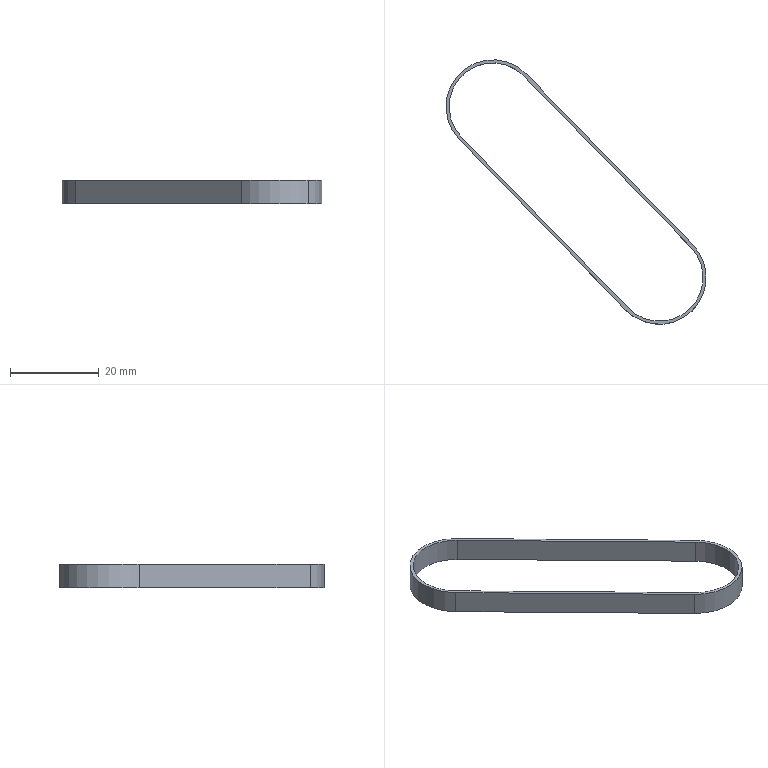Part | SolidWorks | features SplitBody 1 | 1 solid | 12 faces | box 58.599 x 59.577 x 5.25 mm | volume 630.396 mm3 | cylinder 6 | plane 6 | commonest cylinder face diameters 19.677 x3 21.077 x3
STEP:
#1=CARTESIAN_POINT('',(-26.957,211.226,-241.916));
#2=VERTEX_POINT('',#1);
#3=CARTESIAN_POINT('',(-27.136,197.313,-241.916));
#4=VERTEX_POINT('',#3);
#5=CARTESIAN_POINT('',(-34.003,204.359,-241.916));
#6=DIRECTION('',(0.,0.,-1.));
#7=DIRECTION('',(-0.698,0.7161,0.));
#8=AXIS2_PLACEMENT_3D('',#5,#6,#7);
#9=CIRCLE('',#8,9.838);
#10=EDGE_CURVE('',#2,#4,#9,.T.);
#11=ORIENTED_EDGE('',*,*,#10,.T.);
#12=CARTESIAN_POINT('',(-27.136,197.313,-236.666));
#13=VERTEX_POINT('',#12);
#14=CARTESIAN_POINT('',(-27.136,197.313,-241.916));
#15=DIRECTION('',(0.,0.,1.));
#16=VECTOR('',#15,1000.);
#17=LINE('',#14,#16);
#18=EDGE_CURVE('',#4,#13,#17,.T.);
#19=ORIENTED_EDGE('',*,*,#18,.T.);
#20=CARTESIAN_POINT('',(-26.957,211.226,-236.666));
#21=VERTEX_POINT('',#20);
#22=CARTESIAN_POINT('',(-34.003,204.359,-236.666));
#23=DIRECTION('',(0.,0.,-1.));
#24=DIRECTION('',(-0.698,0.7161,0.));
#25=AXIS2_PLACEMENT_3D('',#22,#23,#24);
#26=CIRCLE('',#25,9.838);
#27=EDGE_CURVE('',#21,#13,#26,.T.);
#28=ORIENTED_EDGE('',*,*,#27,.F.);
#29=CARTESIAN_POINT('',(-26.957,211.226,-241.916));
#30=DIRECTION('',(0.,0.,1.));
#31=VECTOR('',#30,1000.);
#32=LINE('',#29,#31);
#33=EDGE_CURVE('',#2,#21,#32,.T.);
#34=ORIENTED_EDGE('',*,*,#33,.F.);
#35=EDGE_LOOP('',(#11,#19,#28,#34));
#36=FACE_OUTER_BOUND('',#35,.T.);
#37=CARTESIAN_POINT('',(-34.003,204.359,-241.916));
#38=DIRECTION('',(0.,0.,1.));
#39=DIRECTION('',(0.698,-0.7161,0.));
#40=AXIS2_PLACEMENT_3D('',#37,#38,#39);
#41=CYLINDRICAL_SURFACE('',#40,9.838);
#42=ADVANCED_FACE('',(#36),#41,.F.);
#43=CARTESIAN_POINT('',(-26.648,196.812,-241.916));
#44=VERTEX_POINT('',#43);
#45=CARTESIAN_POINT('',(-41.55,197.004,-241.916));
#46=VERTEX_POINT('',#45);
#47=CARTESIAN_POINT('',(-34.003,204.359,-241.916));
#48=DIRECTION('',(0.,0.,-1.));
#49=DIRECTION('',(-0.698,0.7161,0.));
#50=AXIS2_PLACEMENT_3D('',#47,#48,#49);
#51=CIRCLE('',#50,10.538);
#52=EDGE_CURVE('',#44,#46,#51,.T.);
#53=ORIENTED_EDGE('',*,*,#52,.F.);
#54=CARTESIAN_POINT('',(-26.648,196.812,-236.666));
#55=VERTEX_POINT('',#54);
#56=CARTESIAN_POINT('',(-26.648,196.812,-241.916));
#57=DIRECTION('',(0.,0.,1.));
#58=VECTOR('',#57,1000.);
#59=LINE('',#56,#58);
#60=EDGE_CURVE('',#44,#55,#59,.T.);
#61=ORIENTED_EDGE('',*,*,#60,.T.);
#62=CARTESIAN_POINT('',(-41.55,197.004,-236.666));
#63=VERTEX_POINT('',#62);
#64=CARTESIAN_POINT('',(-34.003,204.359,-236.666));
#65=DIRECTION('',(0.,0.,-1.));
#66=DIRECTION('',(-0.698,0.7161,0.));
#67=AXIS2_PLACEMENT_3D('',#64,#65,#66);
#68=CIRCLE('',#67,10.538);
#69=EDGE_CURVE('',#55,#63,#68,.T.);
#70=ORIENTED_EDGE('',*,*,#69,.T.);
#71=CARTESIAN_POINT('',(-41.55,197.004,-241.916));
#72=DIRECTION('',(0.,0.,1.));
#73=VECTOR('',#72,1000.);
#74=LINE('',#71,#73);
#75=EDGE_CURVE('',#46,#63,#74,.T.);
#76=ORIENTED_EDGE('',*,*,#75,.F.);
#77=EDGE_LOOP('',(#53,#61,#70,#76));
#78=FACE_OUTER_BOUND('',#77,.T.);
#79=CARTESIAN_POINT('',(-34.003,204.359,-241.916));
#80=DIRECTION('',(0.,0.,1.));
#81=DIRECTION('',(0.698,-0.7161,0.));
#82=AXIS2_PLACEMENT_3D('',#79,#80,#81);
#83=CYLINDRICAL_SURFACE('',#82,10.538);
#84=ADVANCED_FACE('',(#78),#83,.T.);
#85=CARTESIAN_POINT('',(-26.456,211.714,-241.916));
#86=VERTEX_POINT('',#85);
#87=CARTESIAN_POINT('',(-34.003,204.359,-241.916));
#88=DIRECTION('',(0.,0.,-1.));
#89=DIRECTION('',(-0.698,0.7161,0.));
#90=AXIS2_PLACEMENT_3D('',#87,#88,#89);
#91=CIRCLE('',#90,10.538);
#92=EDGE_CURVE('',#86,#44,#91,.T.);
#93=ORIENTED_EDGE('',*,*,#92,.T.);
#94=ORIENTED_EDGE('',*,*,#52,.T.);
#95=CARTESIAN_POINT('',(-79.072,235.504,-241.916));
#96=VERTEX_POINT('',#95);
#97=CARTESIAN_POINT('',(-79.072,235.504,-241.916));
#98=DIRECTION('',(-0.698,0.7161,0.));
#99=VECTOR('',#98,1000.);
#100=LINE('',#97,#99);
#101=EDGE_CURVE('',#46,#96,#100,.T.);
#102=ORIENTED_EDGE('',*,*,#101,.T.);
#103=CARTESIAN_POINT('',(-63.978,250.214,-241.916));
#104=VERTEX_POINT('',#103);
#105=CARTESIAN_POINT('',(-71.525,242.859,-241.916));
#106=DIRECTION('',(0.,0.,-1.));
#107=DIRECTION('',(-0.698,0.7161,0.));
#108=AXIS2_PLACEMENT_3D('',#105,#106,#107);
#109=CIRCLE('',#108,10.538);
#110=EDGE_CURVE('',#96,#104,#109,.T.);
#111=ORIENTED_EDGE('',*,*,#110,.T.);
#112=CARTESIAN_POINT('',(-26.456,211.714,-241.916));
#113=DIRECTION('',(0.698,-0.7161,0.));
#114=VECTOR('',#113,1000.);
#115=LINE('',#112,#114);
#116=EDGE_CURVE('',#104,#86,#115,.T.);
#117=ORIENTED_EDGE('',*,*,#116,.T.);
#118=EDGE_LOOP('',(#93,#94,#102,#111,#117));
#119=FACE_OUTER_BOUND('',#118,.T.);
#120=CARTESIAN_POINT('',(-41.049,197.492,-241.916));
#121=VERTEX_POINT('',#120);
#122=CARTESIAN_POINT('',(-78.57,235.992,-241.916));
#123=VERTEX_POINT('',#122);
#124=CARTESIAN_POINT('',(-78.57,235.992,-241.916));
#125=DIRECTION('',(-0.698,0.7161,0.));
#126=VECTOR('',#125,1000.);
#127=LINE('',#124,#126);
#128=EDGE_CURVE('',#121,#123,#127,.T.);
#129=ORIENTED_EDGE('',*,*,#128,.F.);
#130=CARTESIAN_POINT('',(-34.003,204.359,-241.916));
#131=DIRECTION('',(0.,0.,-1.));
#132=DIRECTION('',(-0.698,0.7161,0.));
#133=AXIS2_PLACEMENT_3D('',#130,#131,#132);
#134=CIRCLE('',#133,9.838);
#135=EDGE_CURVE('',#4,#121,#134,.T.);
#136=ORIENTED_EDGE('',*,*,#135,.F.);
#137=ORIENTED_EDGE('',*,*,#10,.F.);
#138=CARTESIAN_POINT('',(-64.479,249.726,-241.916));
#139=VERTEX_POINT('',#138);
#140=CARTESIAN_POINT('',(-26.957,211.226,-241.916));
#141=DIRECTION('',(0.698,-0.7161,0.));
#142=VECTOR('',#141,1000.);
#143=LINE('',#140,#142);
#144=EDGE_CURVE('',#139,#2,#143,.T.);
#145=ORIENTED_EDGE('',*,*,#144,.F.);
#146=CARTESIAN_POINT('',(-71.525,242.859,-241.916));
#147=DIRECTION('',(0.,0.,-1.));
#148=DIRECTION('',(-0.698,0.7161,0.));
#149=AXIS2_PLACEMENT_3D('',#146,#147,#148);
#150=CIRCLE('',#149,9.838);
#151=EDGE_CURVE('',#123,#139,#150,.T.);
#152=ORIENTED_EDGE('',*,*,#151,.F.);
#153=EDGE_LOOP('',(#129,#136,#137,#145,#152));
#154=FACE_BOUND('',#153,.T.);
#155=CARTESIAN_POINT('',(-34.003,204.359,-241.916));
#156=DIRECTION('',(0.,0.,-1.));
#157=DIRECTION('',(-0.698,0.7161,0.));
#158=AXIS2_PLACEMENT_3D('',#155,#156,#157);
#159=PLANE('',#158);
#160=ADVANCED_FACE('',(#119,#154),#159,.T.);
#161=CARTESIAN_POINT('',(-26.456,211.714,-236.666));
#162=VERTEX_POINT('',#161);
#163=CARTESIAN_POINT('',(-34.003,204.359,-236.666));
#164=DIRECTION('',(0.,0.,-1.));
#165=DIRECTION('',(-0.698,0.7161,0.));
#166=AXIS2_PLACEMENT_3D('',#163,#164,#165);
#167=CIRCLE('',#166,10.538);
#168=EDGE_CURVE('',#162,#55,#167,.T.);
#169=ORIENTED_EDGE('',*,*,#168,.F.);
#170=CARTESIAN_POINT('',(-63.978,250.214,-236.666));
#171=VERTEX_POINT('',#170);
#172=CARTESIAN_POINT('',(-26.456,211.714,-236.666));
#173=DIRECTION('',(0.698,-0.7161,0.));
#174=VECTOR('',#173,1000.);
#175=LINE('',#172,#174);
#176=EDGE_CURVE('',#171,#162,#175,.T.);
#177=ORIENTED_EDGE('',*,*,#176,.F.);
#178=CARTESIAN_POINT('',(-79.072,235.504,-236.666));
#179=VERTEX_POINT('',#178);
#180=CARTESIAN_POINT('',(-71.525,242.859,-236.666));
#181=DIRECTION('',(0.,0.,-1.));
#182=DIRECTION('',(-0.698,0.7161,0.));
#183=AXIS2_PLACEMENT_3D('',#180,#181,#182);
#184=CIRCLE('',#183,10.538);
#185=EDGE_CURVE('',#179,#171,#184,.T.);
#186=ORIENTED_EDGE('',*,*,#185,.F.);
#187=CARTESIAN_POINT('',(-79.072,235.504,-236.666));
#188=DIRECTION('',(-0.698,0.7161,0.));
#189=VECTOR('',#188,1000.);
#190=LINE('',#187,#189);
#191=EDGE_CURVE('',#63,#179,#190,.T.);
#192=ORIENTED_EDGE('',*,*,#191,.F.);
#193=ORIENTED_EDGE('',*,*,#69,.F.);
#194=EDGE_LOOP('',(#169,#177,#186,#192,#193));
#195=FACE_OUTER_BOUND('',#194,.T.);
#196=ORIENTED_EDGE('',*,*,#27,.T.);
#197=CARTESIAN_POINT('',(-41.049,197.492,-236.666));
#198=VERTEX_POINT('',#197);
#199=CARTESIAN_POINT('',(-34.003,204.359,-236.666));
#200=DIRECTION('',(0.,0.,-1.));
#201=DIRECTION('',(-0.698,0.7161,0.));
#202=AXIS2_PLACEMENT_3D('',#199,#200,#201);
#203=CIRCLE('',#202,9.838);
#204=EDGE_CURVE('',#13,#198,#203,.T.);
#205=ORIENTED_EDGE('',*,*,#204,.T.);
#206=CARTESIAN_POINT('',(-78.57,235.992,-236.666));
#207=VERTEX_POINT('',#206);
#208=CARTESIAN_POINT('',(-78.57,235.992,-236.666));
#209=DIRECTION('',(-0.698,0.7161,0.));
#210=VECTOR('',#209,1000.);
#211=LINE('',#208,#210);
#212=EDGE_CURVE('',#198,#207,#211,.T.);
#213=ORIENTED_EDGE('',*,*,#212,.T.);
#214=CARTESIAN_POINT('',(-64.479,249.726,-236.666));
#215=VERTEX_POINT('',#214);
#216=CARTESIAN_POINT('',(-71.525,242.859,-236.666));
#217=DIRECTION('',(0.,0.,-1.));
#218=DIRECTION('',(-0.698,0.7161,0.));
#219=AXIS2_PLACEMENT_3D('',#216,#217,#218);
#220=CIRCLE('',#219,9.838);
#221=EDGE_CURVE('',#207,#215,#220,.T.);
#222=ORIENTED_EDGE('',*,*,#221,.T.);
#223=CARTESIAN_POINT('',(-26.957,211.226,-236.666));
#224=DIRECTION('',(0.698,-0.7161,0.));
#225=VECTOR('',#224,1000.);
#226=LINE('',#223,#225);
#227=EDGE_CURVE('',#215,#21,#226,.T.);
#228=ORIENTED_EDGE('',*,*,#227,.T.);
#229=EDGE_LOOP('',(#196,#205,#213,#222,#228));
#230=FACE_BOUND('',#229,.T.);
#231=CARTESIAN_POINT('',(-34.003,204.359,-236.666));
#232=DIRECTION('',(0.,0.,-1.));
#233=DIRECTION('',(-0.698,0.7161,0.));
#234=AXIS2_PLACEMENT_3D('',#231,#232,#233);
#235=PLANE('',#234);
#236=ADVANCED_FACE('',(#195,#230),#235,.F.);
#237=ORIENTED_EDGE('',*,*,#60,.F.);
#238=ORIENTED_EDGE('',*,*,#92,.F.);
#239=CARTESIAN_POINT('',(-26.456,211.714,-241.916));
#240=DIRECTION('',(0.,0.,1.));
#241=VECTOR('',#240,1000.);
#242=LINE('',#239,#241);
#243=EDGE_CURVE('',#86,#162,#242,.T.);
#244=ORIENTED_EDGE('',*,*,#243,.T.);
#245=ORIENTED_EDGE('',*,*,#168,.T.);
#246=EDGE_LOOP('',(#237,#238,#244,#245));
#247=FACE_OUTER_BOUND('',#246,.T.);
#248=CARTESIAN_POINT('',(-34.003,204.359,-241.916));
#249=DIRECTION('',(0.,0.,1.));
#250=DIRECTION('',(0.698,-0.7161,0.));
#251=AXIS2_PLACEMENT_3D('',#248,#249,#250);
#252=CYLINDRICAL_SURFACE('',#251,10.538);
#253=ADVANCED_FACE('',(#247),#252,.T.);
#254=ORIENTED_EDGE('',*,*,#191,.T.);
#255=CARTESIAN_POINT('',(-79.072,235.504,-241.916));
#256=DIRECTION('',(0.,0.,1.));
#257=VECTOR('',#256,1000.);
#258=LINE('',#255,#257);
#259=EDGE_CURVE('',#96,#179,#258,.T.);
#260=ORIENTED_EDGE('',*,*,#259,.F.);
#261=ORIENTED_EDGE('',*,*,#101,.F.);
#262=ORIENTED_EDGE('',*,*,#75,.T.);
#263=EDGE_LOOP('',(#254,#260,#261,#262));
#264=FACE_OUTER_BOUND('',#263,.T.);
#265=CARTESIAN_POINT('',(-79.072,235.504,-241.916));
#266=DIRECTION('',(0.7161,0.698,0.));
#267=DIRECTION('',(0.698,-0.7161,0.));
#268=AXIS2_PLACEMENT_3D('',#265,#266,#267);
#269=PLANE('',#268);
#270=ADVANCED_FACE('',(#264),#269,.F.);
#271=ORIENTED_EDGE('',*,*,#185,.T.);
#272=CARTESIAN_POINT('',(-63.978,250.214,-241.916));
#273=DIRECTION('',(0.,0.,1.));
#274=VECTOR('',#273,1000.);
#275=LINE('',#272,#274);
#276=EDGE_CURVE('',#104,#171,#275,.T.);
#277=ORIENTED_EDGE('',*,*,#276,.F.);
#278=ORIENTED_EDGE('',*,*,#110,.F.);
#279=ORIENTED_EDGE('',*,*,#259,.T.);
#280=EDGE_LOOP('',(#271,#277,#278,#279));
#281=FACE_OUTER_BOUND('',#280,.T.);
#282=CARTESIAN_POINT('',(-71.525,242.859,-241.916));
#283=DIRECTION('',(0.,0.,1.));
#284=DIRECTION('',(0.698,-0.7161,0.));
#285=AXIS2_PLACEMENT_3D('',#282,#283,#284);
#286=CYLINDRICAL_SURFACE('',#285,10.538);
#287=ADVANCED_FACE('',(#281),#286,.T.);
#288=ORIENTED_EDGE('',*,*,#176,.T.);
#289=ORIENTED_EDGE('',*,*,#243,.F.);
#290=ORIENTED_EDGE('',*,*,#116,.F.);
#291=ORIENTED_EDGE('',*,*,#276,.T.);
#292=EDGE_LOOP('',(#288,#289,#290,#291));
#293=FACE_OUTER_BOUND('',#292,.T.);
#294=CARTESIAN_POINT('',(-26.456,211.714,-241.916));
#295=DIRECTION('',(-0.7161,-0.698,0.));
#296=DIRECTION('',(-0.698,0.7161,0.));
#297=AXIS2_PLACEMENT_3D('',#294,#295,#296);
#298=PLANE('',#297);
#299=ADVANCED_FACE('',(#293),#298,.F.);
#300=ORIENTED_EDGE('',*,*,#18,.F.);
#301=ORIENTED_EDGE('',*,*,#135,.T.);
#302=CARTESIAN_POINT('',(-41.049,197.492,-241.916));
#303=DIRECTION('',(0.,0.,1.));
#304=VECTOR('',#303,1000.);
#305=LINE('',#302,#304);
#306=EDGE_CURVE('',#121,#198,#305,.T.);
#307=ORIENTED_EDGE('',*,*,#306,.T.);
#308=ORIENTED_EDGE('',*,*,#204,.F.);
#309=EDGE_LOOP('',(#300,#301,#307,#308));
#310=FACE_OUTER_BOUND('',#309,.T.);
#311=CARTESIAN_POINT('',(-34.003,204.359,-241.916));
#312=DIRECTION('',(0.,0.,1.));
#313=DIRECTION('',(0.698,-0.7161,0.));
#314=AXIS2_PLACEMENT_3D('',#311,#312,#313);
#315=CYLINDRICAL_SURFACE('',#314,9.838);
#316=ADVANCED_FACE('',(#310),#315,.F.);
#317=ORIENTED_EDGE('',*,*,#212,.F.);
#318=ORIENTED_EDGE('',*,*,#306,.F.);
#319=ORIENTED_EDGE('',*,*,#128,.T.);
#320=CARTESIAN_POINT('',(-78.57,235.992,-241.916));
#321=DIRECTION('',(0.,0.,1.));
#322=VECTOR('',#321,1000.);
#323=LINE('',#320,#322);
#324=EDGE_CURVE('',#123,#207,#323,.T.);
#325=ORIENTED_EDGE('',*,*,#324,.T.);
#326=EDGE_LOOP('',(#317,#318,#319,#325));
#327=FACE_OUTER_BOUND('',#326,.T.);
#328=CARTESIAN_POINT('',(-78.57,235.992,-241.916));
#329=DIRECTION('',(0.7161,0.698,0.));
#330=DIRECTION('',(0.698,-0.7161,0.));
#331=AXIS2_PLACEMENT_3D('',#328,#329,#330);
#332=PLANE('',#331);
#333=ADVANCED_FACE('',(#327),#332,.T.);
#334=ORIENTED_EDGE('',*,*,#221,.F.);
#335=ORIENTED_EDGE('',*,*,#324,.F.);
#336=ORIENTED_EDGE('',*,*,#151,.T.);
#337=CARTESIAN_POINT('',(-64.479,249.726,-241.916));
#338=DIRECTION('',(0.,0.,1.));
#339=VECTOR('',#338,1000.);
#340=LINE('',#337,#339);
#341=EDGE_CURVE('',#139,#215,#340,.T.);
#342=ORIENTED_EDGE('',*,*,#341,.T.);
#343=EDGE_LOOP('',(#334,#335,#336,#342));
#344=FACE_OUTER_BOUND('',#343,.T.);
#345=CARTESIAN_POINT('',(-71.525,242.859,-241.916));
#346=DIRECTION('',(0.,0.,1.));
#347=DIRECTION('',(0.698,-0.7161,0.));
#348=AXIS2_PLACEMENT_3D('',#345,#346,#347);
#349=CYLINDRICAL_SURFACE('',#348,9.838);
#350=ADVANCED_FACE('',(#344),#349,.F.);
#351=ORIENTED_EDGE('',*,*,#227,.F.);
#352=ORIENTED_EDGE('',*,*,#341,.F.);
#353=ORIENTED_EDGE('',*,*,#144,.T.);
#354=ORIENTED_EDGE('',*,*,#33,.T.);
#355=EDGE_LOOP('',(#351,#352,#353,#354));
#356=FACE_OUTER_BOUND('',#355,.T.);
#357=CARTESIAN_POINT('',(-26.957,211.226,-241.916));
#358=DIRECTION('',(-0.7161,-0.698,0.));
#359=DIRECTION('',(-0.698,0.7161,0.));
#360=AXIS2_PLACEMENT_3D('',#357,#358,#359);
#361=PLANE('',#360);
#362=ADVANCED_FACE('',(#356),#361,.T.);
#363=CLOSED_SHELL('',(#42,#84,#160,#236,#253,#270,#287,#299,#316,#333,#350,#362));
#364=MANIFOLD_SOLID_BREP('',#363);
#365=CARTESIAN_POINT('',(0.,0.,0.));
#366=DIRECTION('',(0.,0.,1.));
#367=DIRECTION('',(1.,0.,0.));
#368=AXIS2_PLACEMENT_3D('',#365,#366,#367);
#369=(LENGTH_UNIT()NAMED_UNIT(*)SI_UNIT(.MILLI.,.METRE.));
#370=UNCERTAINTY_MEASURE_WITH_UNIT(LENGTH_MEASURE(0.00001),#369,'','');
#371=(NAMED_UNIT(*)PLANE_ANGLE_UNIT()SI_UNIT($,.RADIAN.));
#372=(NAMED_UNIT(*)SI_UNIT($,.STERADIAN.)SOLID_ANGLE_UNIT());
#373=(GEOMETRIC_REPRESENTATION_CONTEXT(3)GLOBAL_UNCERTAINTY_ASSIGNED_CONTEXT((#370))GLOBAL_UNIT_ASSIGNED_CONTEXT((#369,#371,#372))REPRESENTATION_CONTEXT('',''));
#374=ADVANCED_BREP_SHAPE_REPRESENTATION('',(#364,#368),#373);